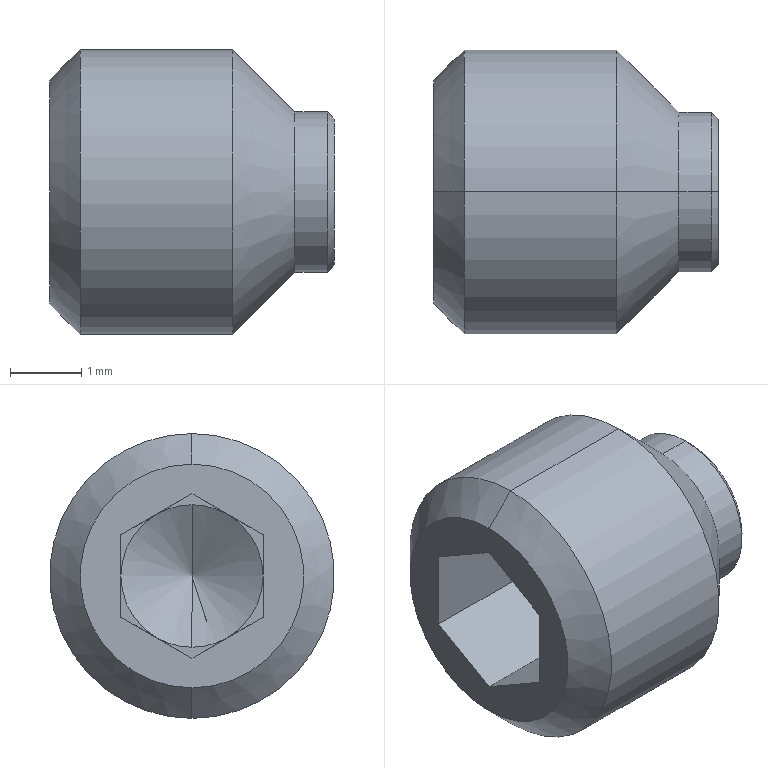Part | NX | features BREP 1 | 1 solid | 26 faces | box 4 x 4 x 4 mm | volume 34.482 mm3 | plane 14 | cone 8 | cylinder 4 | commonest cylinder face diameters 2.25 x2 4 x2